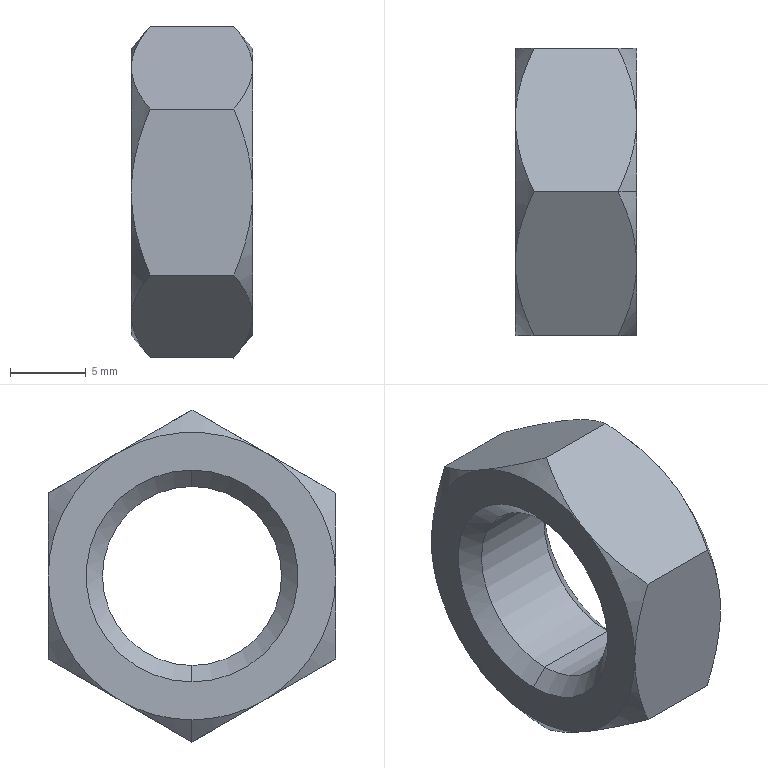Part | SolidWorks | features BaseBody 1 | 1 solid | 28 faces | box 8 x 19 x 21.939 mm | volume 1553 mm3 | cone 18 | plane 8 | cylinder 2 | commonest cylinder face diameters 11.835 x2
STEP:
#1=CARTESIAN_POINT('',(2.917,0.,-5.918));
#2=VERTEX_POINT('',#1);
#3=CARTESIAN_POINT('',(2.917,0.,5.918));
#4=VERTEX_POINT('',#3);
#5=CARTESIAN_POINT('',(2.917,0.,0.));
#6=DIRECTION('',(-1.,0.,0.));
#7=DIRECTION('',(0.,0.,1.));
#8=AXIS2_PLACEMENT_3D('',#5,#6,#7);
#9=CIRCLE('',#8,5.918);
#10=EDGE_CURVE('',#2,#4,#9,.T.);
#11=ORIENTED_EDGE('',*,*,#10,.F.);
#12=CARTESIAN_POINT('',(-2.917,0.,-5.918));
#13=VERTEX_POINT('',#12);
#14=CARTESIAN_POINT('',(4.,0.,-5.918));
#15=DIRECTION('',(-1.,0.,0.));
#16=VECTOR('',#15,1000.);
#17=LINE('',#14,#16);
#18=EDGE_CURVE('',#2,#13,#17,.T.);
#19=ORIENTED_EDGE('',*,*,#18,.T.);
#20=CARTESIAN_POINT('',(-2.917,0.,5.918));
#21=VERTEX_POINT('',#20);
#22=CARTESIAN_POINT('',(-2.917,0.,0.));
#23=DIRECTION('',(1.,0.,0.));
#24=DIRECTION('',(0.,0.,1.));
#25=AXIS2_PLACEMENT_3D('',#22,#23,#24);
#26=CIRCLE('',#25,5.918);
#27=EDGE_CURVE('',#21,#13,#26,.T.);
#28=ORIENTED_EDGE('',*,*,#27,.F.);
#29=CARTESIAN_POINT('',(4.,0.,5.918));
#30=DIRECTION('',(-1.,0.,0.));
#31=VECTOR('',#30,1000.);
#32=LINE('',#29,#31);
#33=EDGE_CURVE('',#4,#21,#32,.T.);
#34=ORIENTED_EDGE('',*,*,#33,.F.);
#35=EDGE_LOOP('',(#11,#19,#28,#34));
#36=FACE_OUTER_BOUND('',#35,.T.);
#37=CARTESIAN_POINT('',(4.,0.,0.));
#38=DIRECTION('',(-1.,0.,0.));
#39=DIRECTION('',(0.,0.,1.));
#40=AXIS2_PLACEMENT_3D('',#37,#38,#39);
#41=CYLINDRICAL_SURFACE('',#40,5.918);
#42=ADVANCED_FACE('',(#36),#41,.F.);
#43=ORIENTED_EDGE('',*,*,#27,.T.);
#44=CARTESIAN_POINT('',(-4.,0.,-7.));
#45=VERTEX_POINT('',#44);
#46=CARTESIAN_POINT('',(-4.,0.,-7.));
#47=DIRECTION('',(-0.7071,0.,-0.7071));
#48=VECTOR('',#47,1000.);
#49=LINE('',#46,#48);
#50=EDGE_CURVE('',#13,#45,#49,.T.);
#51=ORIENTED_EDGE('',*,*,#50,.T.);
#52=CARTESIAN_POINT('',(-4.,0.,7.));
#53=VERTEX_POINT('',#52);
#54=CARTESIAN_POINT('',(-4.,0.,0.));
#55=DIRECTION('',(1.,0.,0.));
#56=DIRECTION('',(0.,0.,1.));
#57=AXIS2_PLACEMENT_3D('',#54,#55,#56);
#58=CIRCLE('',#57,7.);
#59=EDGE_CURVE('',#53,#45,#58,.T.);
#60=ORIENTED_EDGE('',*,*,#59,.F.);
#61=CARTESIAN_POINT('',(-4.,0.,7.));
#62=DIRECTION('',(-0.7071,0.,0.7071));
#63=VECTOR('',#62,1000.);
#64=LINE('',#61,#63);
#65=EDGE_CURVE('',#21,#53,#64,.T.);
#66=ORIENTED_EDGE('',*,*,#65,.F.);
#67=EDGE_LOOP('',(#43,#51,#60,#66));
#68=FACE_OUTER_BOUND('',#67,.T.);
#69=CARTESIAN_POINT('',(-4.,0.,0.));
#70=DIRECTION('',(-1.,0.,0.));
#71=DIRECTION('',(0.,0.,1.));
#72=AXIS2_PLACEMENT_3D('',#69,#70,#71);
#73=CONICAL_SURFACE('',#72,7.,0.7854);
#74=ADVANCED_FACE('',(#68),#73,.F.);
#75=ORIENTED_EDGE('',*,*,#10,.T.);
#76=CARTESIAN_POINT('',(4.,0.,7.));
#77=VERTEX_POINT('',#76);
#78=CARTESIAN_POINT('',(4.,0.,7.));
#79=DIRECTION('',(0.7071,0.,0.7071));
#80=VECTOR('',#79,1000.);
#81=LINE('',#78,#80);
#82=EDGE_CURVE('',#4,#77,#81,.T.);
#83=ORIENTED_EDGE('',*,*,#82,.T.);
#84=CARTESIAN_POINT('',(4.,0.,-7.));
#85=VERTEX_POINT('',#84);
#86=CARTESIAN_POINT('',(4.,0.,0.));
#87=DIRECTION('',(-1.,0.,0.));
#88=DIRECTION('',(0.,0.,-1.));
#89=AXIS2_PLACEMENT_3D('',#86,#87,#88);
#90=CIRCLE('',#89,7.);
#91=EDGE_CURVE('',#85,#77,#90,.T.);
#92=ORIENTED_EDGE('',*,*,#91,.F.);
#93=CARTESIAN_POINT('',(4.,0.,-7.));
#94=DIRECTION('',(0.7071,0.,-0.7071));
#95=VECTOR('',#94,1000.);
#96=LINE('',#93,#95);
#97=EDGE_CURVE('',#2,#85,#96,.T.);
#98=ORIENTED_EDGE('',*,*,#97,.F.);
#99=EDGE_LOOP('',(#75,#83,#92,#98));
#100=FACE_OUTER_BOUND('',#99,.T.);
#101=CARTESIAN_POINT('',(4.,0.,0.));
#102=DIRECTION('',(1.,0.,0.));
#103=DIRECTION('',(0.,0.,-1.));
#104=AXIS2_PLACEMENT_3D('',#101,#102,#103);
#105=CONICAL_SURFACE('',#104,7.,0.7854);
#106=ADVANCED_FACE('',(#100),#105,.F.);
#107=CARTESIAN_POINT('',(-4.,0.,-9.5));
#108=VERTEX_POINT('',#107);
#109=CARTESIAN_POINT('',(-4.,-4.75,-8.227));
#110=VERTEX_POINT('',#109);
#111=CARTESIAN_POINT('',(-4.,0.,0.));
#112=DIRECTION('',(-1.,0.,0.));
#113=DIRECTION('',(0.,0.,-1.));
#114=AXIS2_PLACEMENT_3D('',#111,#112,#113);
#115=CIRCLE('',#114,9.5);
#116=EDGE_CURVE('',#108,#110,#115,.T.);
#117=ORIENTED_EDGE('',*,*,#116,.F.);
#118=CARTESIAN_POINT('',(-2.767,0.000000009,-10.97));
#119=VERTEX_POINT('',#118);
#120=CARTESIAN_POINT('',(-2.759,0.,-10.978));
#121=DIRECTION('',(0.6428,0.,-0.766));
#122=VECTOR('',#121,1000.);
#123=LINE('',#120,#122);
#124=EDGE_CURVE('',#108,#119,#123,.T.);
#125=ORIENTED_EDGE('',*,*,#124,.T.);
#126=CARTESIAN_POINT('',(-2.767,0.000000009,-10.97));
#127=CARTESIAN_POINT('',(-3.503,-1.52,-10.092));
#128=CARTESIAN_POINT('',(-4.,-3.087,-9.188));
#129=CARTESIAN_POINT('',(-4.,-4.75,-8.227));
#130=B_SPLINE_CURVE_WITH_KNOTS('',3,(#126,#127,#128,#129),.UNSPECIFIED.,.F.,.F.,(4,4),(0.,0.005622),.UNSPECIFIED.);
#131=EDGE_CURVE('',#119,#110,#130,.T.);
#132=ORIENTED_EDGE('',*,*,#131,.T.);
#133=EDGE_LOOP('',(#117,#125,#132));
#134=FACE_OUTER_BOUND('',#133,.T.);
#135=CARTESIAN_POINT('',(-2.759,0.,0.));
#136=DIRECTION('',(1.,0.,0.));
#137=DIRECTION('',(0.,0.,-1.));
#138=AXIS2_PLACEMENT_3D('',#135,#136,#137);
#139=CONICAL_SURFACE('',#138,10.978,0.8727);
#140=ADVANCED_FACE('',(#134),#139,.T.);
#141=CARTESIAN_POINT('',(4.,0.,9.5));
#142=VERTEX_POINT('',#141);
#143=CARTESIAN_POINT('',(4.,-4.75,8.227));
#144=VERTEX_POINT('',#143);
#145=CARTESIAN_POINT('',(4.,0.,0.));
#146=DIRECTION('',(1.,0.,0.));
#147=DIRECTION('',(0.,0.,1.));
#148=AXIS2_PLACEMENT_3D('',#145,#146,#147);
#149=CIRCLE('',#148,9.5);
#150=EDGE_CURVE('',#142,#144,#149,.T.);
#151=ORIENTED_EDGE('',*,*,#150,.F.);
#152=CARTESIAN_POINT('',(2.767,0.000000009,10.97));
#153=VERTEX_POINT('',#152);
#154=CARTESIAN_POINT('',(2.759,0.,10.978));
#155=DIRECTION('',(-0.6428,0.,0.766));
#156=VECTOR('',#155,1000.);
#157=LINE('',#154,#156);
#158=EDGE_CURVE('',#142,#153,#157,.T.);
#159=ORIENTED_EDGE('',*,*,#158,.T.);
#160=CARTESIAN_POINT('',(2.767,0.000000009,10.97));
#161=CARTESIAN_POINT('',(3.503,-1.52,10.092));
#162=CARTESIAN_POINT('',(4.,-3.087,9.188));
#163=CARTESIAN_POINT('',(4.,-4.75,8.227));
#164=B_SPLINE_CURVE_WITH_KNOTS('',3,(#160,#161,#162,#163),.UNSPECIFIED.,.F.,.F.,(4,4),(0.,0.005622),.UNSPECIFIED.);
#165=EDGE_CURVE('',#153,#144,#164,.T.);
#166=ORIENTED_EDGE('',*,*,#165,.T.);
#167=EDGE_LOOP('',(#151,#159,#166));
#168=FACE_OUTER_BOUND('',#167,.T.);
#169=CARTESIAN_POINT('',(2.759,0.,0.));
#170=DIRECTION('',(-1.,0.,0.));
#171=DIRECTION('',(0.,0.,1.));
#172=AXIS2_PLACEMENT_3D('',#169,#170,#171);
#173=CONICAL_SURFACE('',#172,10.978,0.8727);
#174=ADVANCED_FACE('',(#168),#173,.T.);
#175=ORIENTED_EDGE('',*,*,#18,.F.);
#176=CARTESIAN_POINT('',(2.917,0.,0.));
#177=DIRECTION('',(-1.,0.,0.));
#178=DIRECTION('',(0.,0.,1.));
#179=AXIS2_PLACEMENT_3D('',#176,#177,#178);
#180=CIRCLE('',#179,5.918);
#181=EDGE_CURVE('',#4,#2,#180,.T.);
#182=ORIENTED_EDGE('',*,*,#181,.F.);
#183=ORIENTED_EDGE('',*,*,#33,.T.);
#184=CARTESIAN_POINT('',(-2.917,0.,0.));
#185=DIRECTION('',(1.,0.,0.));
#186=DIRECTION('',(0.,0.,1.));
#187=AXIS2_PLACEMENT_3D('',#184,#185,#186);
#188=CIRCLE('',#187,5.918);
#189=EDGE_CURVE('',#13,#21,#188,.T.);
#190=ORIENTED_EDGE('',*,*,#189,.F.);
#191=EDGE_LOOP('',(#175,#182,#183,#190));
#192=FACE_OUTER_BOUND('',#191,.T.);
#193=CARTESIAN_POINT('',(4.,0.,0.));
#194=DIRECTION('',(-1.,0.,0.));
#195=DIRECTION('',(0.,0.,1.));
#196=AXIS2_PLACEMENT_3D('',#193,#194,#195);
#197=CYLINDRICAL_SURFACE('',#196,5.918);
#198=ADVANCED_FACE('',(#192),#197,.F.);
#199=ORIENTED_EDGE('',*,*,#50,.F.);
#200=ORIENTED_EDGE('',*,*,#189,.T.);
#201=ORIENTED_EDGE('',*,*,#65,.T.);
#202=CARTESIAN_POINT('',(-4.,0.,0.));
#203=DIRECTION('',(1.,0.,0.));
#204=DIRECTION('',(0.,0.,1.));
#205=AXIS2_PLACEMENT_3D('',#202,#203,#204);
#206=CIRCLE('',#205,7.);
#207=EDGE_CURVE('',#45,#53,#206,.T.);
#208=ORIENTED_EDGE('',*,*,#207,.F.);
#209=EDGE_LOOP('',(#199,#200,#201,#208));
#210=FACE_OUTER_BOUND('',#209,.T.);
#211=CARTESIAN_POINT('',(-4.,0.,0.));
#212=DIRECTION('',(-1.,0.,0.));
#213=DIRECTION('',(0.,0.,1.));
#214=AXIS2_PLACEMENT_3D('',#211,#212,#213);
#215=CONICAL_SURFACE('',#214,7.,0.7854);
#216=ADVANCED_FACE('',(#210),#215,.F.);
#217=ORIENTED_EDGE('',*,*,#82,.F.);
#218=ORIENTED_EDGE('',*,*,#181,.T.);
#219=ORIENTED_EDGE('',*,*,#97,.T.);
#220=CARTESIAN_POINT('',(4.,0.,0.));
#221=DIRECTION('',(-1.,0.,0.));
#222=DIRECTION('',(0.,0.,-1.));
#223=AXIS2_PLACEMENT_3D('',#220,#221,#222);
#224=CIRCLE('',#223,7.);
#225=EDGE_CURVE('',#77,#85,#224,.T.);
#226=ORIENTED_EDGE('',*,*,#225,.F.);
#227=EDGE_LOOP('',(#217,#218,#219,#226));
#228=FACE_OUTER_BOUND('',#227,.T.);
#229=CARTESIAN_POINT('',(4.,0.,0.));
#230=DIRECTION('',(1.,0.,0.));
#231=DIRECTION('',(0.,0.,-1.));
#232=AXIS2_PLACEMENT_3D('',#229,#230,#231);
#233=CONICAL_SURFACE('',#232,7.,0.7854);
#234=ADVANCED_FACE('',(#228),#233,.F.);
#235=CARTESIAN_POINT('',(-4.,-9.5,0.));
#236=VERTEX_POINT('',#235);
#237=CARTESIAN_POINT('',(-4.,-4.75,8.227));
#238=VERTEX_POINT('',#237);
#239=CARTESIAN_POINT('',(-4.,0.,0.));
#240=DIRECTION('',(-1.,0.,0.));
#241=DIRECTION('',(0.,1.,0.));
#242=AXIS2_PLACEMENT_3D('',#239,#240,#241);
#243=CIRCLE('',#242,9.5);
#244=EDGE_CURVE('',#236,#238,#243,.T.);
#245=ORIENTED_EDGE('',*,*,#244,.T.);
#246=CARTESIAN_POINT('',(-4.,4.75,8.227));
#247=VERTEX_POINT('',#246);
#248=CARTESIAN_POINT('',(-4.,0.,0.));
#249=DIRECTION('',(-1.,0.,0.));
#250=DIRECTION('',(0.,0.,-1.));
#251=AXIS2_PLACEMENT_3D('',#248,#249,#250);
#252=CIRCLE('',#251,9.5);
#253=EDGE_CURVE('',#238,#247,#252,.T.);
#254=ORIENTED_EDGE('',*,*,#253,.T.);
#255=CARTESIAN_POINT('',(-4.,9.5,0.));
#256=VERTEX_POINT('',#255);
#257=CARTESIAN_POINT('',(-4.,0.,0.));
#258=DIRECTION('',(-1.,0.,0.));
#259=DIRECTION('',(0.,0.,-1.));
#260=AXIS2_PLACEMENT_3D('',#257,#258,#259);
#261=CIRCLE('',#260,9.5);
#262=EDGE_CURVE('',#247,#256,#261,.T.);
#263=ORIENTED_EDGE('',*,*,#262,.T.);
#264=CARTESIAN_POINT('',(-4.,4.75,-8.227));
#265=VERTEX_POINT('',#264);
#266=CARTESIAN_POINT('',(-4.,0.,0.));
#267=DIRECTION('',(-1.,0.,0.));
#268=DIRECTION('',(0.,1.,0.));
#269=AXIS2_PLACEMENT_3D('',#266,#267,#268);
#270=CIRCLE('',#269,9.5);
#271=EDGE_CURVE('',#256,#265,#270,.T.);
#272=ORIENTED_EDGE('',*,*,#271,.T.);
#273=CARTESIAN_POINT('',(-4.,0.,0.));
#274=DIRECTION('',(-1.,0.,0.));
#275=DIRECTION('',(0.,0.,-1.));
#276=AXIS2_PLACEMENT_3D('',#273,#274,#275);
#277=CIRCLE('',#276,9.5);
#278=EDGE_CURVE('',#265,#108,#277,.T.);
#279=ORIENTED_EDGE('',*,*,#278,.T.);
#280=ORIENTED_EDGE('',*,*,#116,.T.);
#281=CARTESIAN_POINT('',(-4.,0.,0.));
#282=DIRECTION('',(-1.,0.,0.));
#283=DIRECTION('',(0.,0.,-1.));
#284=AXIS2_PLACEMENT_3D('',#281,#282,#283);
#285=CIRCLE('',#284,9.5);
#286=EDGE_CURVE('',#110,#236,#285,.T.);
#287=ORIENTED_EDGE('',*,*,#286,.T.);
#288=EDGE_LOOP('',(#245,#254,#263,#272,#279,#280,#287));
#289=FACE_OUTER_BOUND('',#288,.T.);
#290=ORIENTED_EDGE('',*,*,#59,.T.);
#291=ORIENTED_EDGE('',*,*,#207,.T.);
#292=EDGE_LOOP('',(#290,#291));
#293=FACE_BOUND('',#292,.T.);
#294=CARTESIAN_POINT('',(-4.,9.5,0.));
#295=DIRECTION('',(-1.,0.,0.));
#296=DIRECTION('',(0.,0.,1.));
#297=AXIS2_PLACEMENT_3D('',#294,#295,#296);
#298=PLANE('',#297);
#299=ADVANCED_FACE('',(#289,#293),#298,.T.);
#300=ORIENTED_EDGE('',*,*,#91,.T.);
#301=ORIENTED_EDGE('',*,*,#225,.T.);
#302=EDGE_LOOP('',(#300,#301));
#303=FACE_BOUND('',#302,.T.);
#304=CARTESIAN_POINT('',(4.,-9.5,0.));
#305=VERTEX_POINT('',#304);
#306=CARTESIAN_POINT('',(4.,-4.75,-8.227));
#307=VERTEX_POINT('',#306);
#308=CARTESIAN_POINT('',(4.,0.,0.));
#309=DIRECTION('',(1.,0.,0.));
#310=DIRECTION('',(0.,0.,1.));
#311=AXIS2_PLACEMENT_3D('',#308,#309,#310);
#312=CIRCLE('',#311,9.5);
#313=EDGE_CURVE('',#305,#307,#312,.T.);
#314=ORIENTED_EDGE('',*,*,#313,.T.);
#315=CARTESIAN_POINT('',(4.,4.75,-8.227));
#316=VERTEX_POINT('',#315);
#317=CARTESIAN_POINT('',(4.,0.,0.));
#318=DIRECTION('',(1.,0.,0.));
#319=DIRECTION('',(0.,0.,1.));
#320=AXIS2_PLACEMENT_3D('',#317,#318,#319);
#321=CIRCLE('',#320,9.5);
#322=EDGE_CURVE('',#307,#316,#321,.T.);
#323=ORIENTED_EDGE('',*,*,#322,.T.);
#324=CARTESIAN_POINT('',(4.,9.5,0.));
#325=VERTEX_POINT('',#324);
#326=CARTESIAN_POINT('',(4.,0.,0.));
#327=DIRECTION('',(1.,0.,0.));
#328=DIRECTION('',(0.,0.,1.));
#329=AXIS2_PLACEMENT_3D('',#326,#327,#328);
#330=CIRCLE('',#329,9.5);
#331=EDGE_CURVE('',#316,#325,#330,.T.);
#332=ORIENTED_EDGE('',*,*,#331,.T.);
#333=CARTESIAN_POINT('',(4.,4.75,8.227));
#334=VERTEX_POINT('',#333);
#335=CARTESIAN_POINT('',(4.,0.,0.));
#336=DIRECTION('',(1.,0.,0.));
#337=DIRECTION('',(0.,0.,1.));
#338=AXIS2_PLACEMENT_3D('',#335,#336,#337);
#339=CIRCLE('',#338,9.5);
#340=EDGE_CURVE('',#325,#334,#339,.T.);
#341=ORIENTED_EDGE('',*,*,#340,.T.);
#342=CARTESIAN_POINT('',(4.,0.,0.));
#343=DIRECTION('',(1.,0.,0.));
#344=DIRECTION('',(0.,0.,1.));
#345=AXIS2_PLACEMENT_3D('',#342,#343,#344);
#346=CIRCLE('',#345,9.5);
#347=EDGE_CURVE('',#334,#142,#346,.T.);
#348=ORIENTED_EDGE('',*,*,#347,.T.);
#349=ORIENTED_EDGE('',*,*,#150,.T.);
#350=CARTESIAN_POINT('',(4.,0.,0.));
#351=DIRECTION('',(1.,0.,0.));
#352=DIRECTION('',(0.,0.,1.));
#353=AXIS2_PLACEMENT_3D('',#350,#351,#352);
#354=CIRCLE('',#353,9.5);
#355=EDGE_CURVE('',#144,#305,#354,.T.);
#356=ORIENTED_EDGE('',*,*,#355,.T.);
#357=EDGE_LOOP('',(#314,#323,#332,#341,#348,#349,#356));
#358=FACE_OUTER_BOUND('',#357,.T.);
#359=CARTESIAN_POINT('',(4.,7.,0.));
#360=DIRECTION('',(1.,0.,0.));
#361=DIRECTION('',(0.,0.,-1.));
#362=AXIS2_PLACEMENT_3D('',#359,#360,#361);
#363=PLANE('',#362);
#364=ADVANCED_FACE('',(#303,#358),#363,.T.);
#365=ORIENTED_EDGE('',*,*,#253,.F.);
#366=CARTESIAN_POINT('',(-2.767,0.000000018,10.97));
#367=VERTEX_POINT('',#366);
#368=CARTESIAN_POINT('',(-4.,-4.75,8.227));
#369=CARTESIAN_POINT('',(-4.,-3.926,8.703));
#370=CARTESIAN_POINT('',(-3.879,-3.12,9.168));
#371=CARTESIAN_POINT('',(-3.445,-1.537,10.083));
#372=CARTESIAN_POINT('',(-3.134,-0.7569,10.533));
#373=CARTESIAN_POINT('',(-2.767,0.000000018,10.97));
#374=B_SPLINE_CURVE_WITH_KNOTS('',3,(#368,#369,#370,#371,#372,#373),.UNSPECIFIED.,.F.,.F.,(4,2,4),(0.,0.002813,0.005627),.UNSPECIFIED.);
#375=EDGE_CURVE('',#238,#367,#374,.T.);
#376=ORIENTED_EDGE('',*,*,#375,.T.);
#377=CARTESIAN_POINT('',(-2.767,0.000000018,10.97));
#378=CARTESIAN_POINT('',(-3.503,1.52,10.092));
#379=CARTESIAN_POINT('',(-4.,3.087,9.188));
#380=CARTESIAN_POINT('',(-4.,4.75,8.227));
#381=B_SPLINE_CURVE_WITH_KNOTS('',3,(#377,#378,#379,#380),.UNSPECIFIED.,.F.,.F.,(4,4),(0.,0.005622),.UNSPECIFIED.);
#382=EDGE_CURVE('',#367,#247,#381,.T.);
#383=ORIENTED_EDGE('',*,*,#382,.T.);
#384=EDGE_LOOP('',(#365,#376,#383));
#385=FACE_OUTER_BOUND('',#384,.T.);
#386=CARTESIAN_POINT('',(-2.759,0.,0.));
#387=DIRECTION('',(1.,0.,0.));
#388=DIRECTION('',(0.,0.,-1.));
#389=AXIS2_PLACEMENT_3D('',#386,#387,#388);
#390=CONICAL_SURFACE('',#389,10.978,0.8727);
#391=ADVANCED_FACE('',(#385),#390,.T.);
#392=CARTESIAN_POINT('',(-2.767,-9.5,5.485));
#393=VERTEX_POINT('',#392);
#394=CARTESIAN_POINT('',(-2.767,-9.5,5.485));
#395=CARTESIAN_POINT('',(-3.503,-7.98,6.362));
#396=CARTESIAN_POINT('',(-4.,-6.413,7.267));
#397=CARTESIAN_POINT('',(-4.,-4.75,8.227));
#398=B_SPLINE_CURVE_WITH_KNOTS('',3,(#394,#395,#396,#397),.UNSPECIFIED.,.F.,.F.,(4,4),(0.,0.005622),.UNSPECIFIED.);
#399=EDGE_CURVE('',#393,#238,#398,.T.);
#400=ORIENTED_EDGE('',*,*,#399,.T.);
#401=ORIENTED_EDGE('',*,*,#244,.F.);
#402=CARTESIAN_POINT('',(-4.,-9.5,0.));
#403=CARTESIAN_POINT('',(-4.,-9.5,0.9511));
#404=CARTESIAN_POINT('',(-3.879,-9.5,1.882));
#405=CARTESIAN_POINT('',(-3.445,-9.5,3.711));
#406=CARTESIAN_POINT('',(-3.134,-9.5,4.611));
#407=CARTESIAN_POINT('',(-2.767,-9.5,5.485));
#408=B_SPLINE_CURVE_WITH_KNOTS('',3,(#402,#403,#404,#405,#406,#407),.UNSPECIFIED.,.F.,.F.,(4,2,4),(0.,0.002813,0.005627),.UNSPECIFIED.);
#409=EDGE_CURVE('',#236,#393,#408,.T.);
#410=ORIENTED_EDGE('',*,*,#409,.T.);
#411=EDGE_LOOP('',(#400,#401,#410));
#412=FACE_OUTER_BOUND('',#411,.T.);
#413=CARTESIAN_POINT('',(-2.759,0.,0.));
#414=DIRECTION('',(1.,0.,0.));
#415=DIRECTION('',(0.,1.,0.));
#416=AXIS2_PLACEMENT_3D('',#413,#414,#415);
#417=CONICAL_SURFACE('',#416,10.978,0.8727);
#418=ADVANCED_FACE('',(#412),#417,.T.);
#419=CARTESIAN_POINT('',(-2.767,-9.5,-5.485));
#420=VERTEX_POINT('',#419);
#421=CARTESIAN_POINT('',(-2.767,-9.5,-5.485));
#422=CARTESIAN_POINT('',(-3.503,-9.5,-3.73));
#423=CARTESIAN_POINT('',(-4.,-9.5,-1.921));
#424=CARTESIAN_POINT('',(-4.,-9.5,0.));
#425=B_SPLINE_CURVE_WITH_KNOTS('',3,(#421,#422,#423,#424),.UNSPECIFIED.,.F.,.F.,(4,4),(0.,0.005622),.UNSPECIFIED.);
#426=EDGE_CURVE('',#420,#236,#425,.T.);
#427=ORIENTED_EDGE('',*,*,#426,.T.);
#428=ORIENTED_EDGE('',*,*,#286,.F.);
#429=CARTESIAN_POINT('',(-4.,-4.75,-8.227));
#430=CARTESIAN_POINT('',(-4.,-5.574,-7.752));
#431=CARTESIAN_POINT('',(-3.879,-6.38,-7.286));
#432=CARTESIAN_POINT('',(-3.445,-7.963,-6.372));
#433=CARTESIAN_POINT('',(-3.134,-8.743,-5.922));
#434=CARTESIAN_POINT('',(-2.767,-9.5,-5.485));
#435=B_SPLINE_CURVE_WITH_KNOTS('',3,(#429,#430,#431,#432,#433,#434),.UNSPECIFIED.,.F.,.F.,(4,2,4),(0.,0.002813,0.005627),.UNSPECIFIED.);
#436=EDGE_CURVE('',#110,#420,#435,.T.);
#437=ORIENTED_EDGE('',*,*,#436,.T.);
#438=EDGE_LOOP('',(#427,#428,#437));
#439=FACE_OUTER_BOUND('',#438,.T.);
#440=CARTESIAN_POINT('',(-2.759,0.,0.));
#441=DIRECTION('',(1.,0.,0.));
#442=DIRECTION('',(0.,0.,-1.));
#443=AXIS2_PLACEMENT_3D('',#440,#441,#442);
#444=CONICAL_SURFACE('',#443,10.978,0.8727);
#445=ADVANCED_FACE('',(#439),#444,.T.);
#446=ORIENTED_EDGE('',*,*,#124,.F.);
#447=ORIENTED_EDGE('',*,*,#278,.F.);
#448=CARTESIAN_POINT('',(-4.,4.75,-8.227));
#449=CARTESIAN_POINT('',(-4.,3.926,-8.703));
#450=CARTESIAN_POINT('',(-3.879,3.12,-9.168));
#451=CARTESIAN_POINT('',(-3.445,1.537,-10.083));
#452=CARTESIAN_POINT('',(-3.134,0.7569,-10.533));
#453=CARTESIAN_POINT('',(-2.767,0.000000009,-10.97));
#454=B_SPLINE_CURVE_WITH_KNOTS('',3,(#448,#449,#450,#451,#452,#453),.UNSPECIFIED.,.F.,.F.,(4,2,4),(0.,0.002813,0.005627),.UNSPECIFIED.);
#455=EDGE_CURVE('',#265,#119,#454,.T.);
#456=ORIENTED_EDGE('',*,*,#455,.T.);
#457=EDGE_LOOP('',(#446,#447,#456));
#458=FACE_OUTER_BOUND('',#457,.T.);
#459=CARTESIAN_POINT('',(-2.759,0.,0.));
#460=DIRECTION('',(1.,0.,0.));
#461=DIRECTION('',(0.,0.,-1.));
#462=AXIS2_PLACEMENT_3D('',#459,#460,#461);
#463=CONICAL_SURFACE('',#462,10.978,0.8727);
#464=ADVANCED_FACE('',(#458),#463,.T.);
#465=ORIENTED_EDGE('',*,*,#271,.F.);
#466=CARTESIAN_POINT('',(-2.767,9.5,-5.485));
#467=VERTEX_POINT('',#466);
#468=CARTESIAN_POINT('',(-4.,9.5,0.));
#469=CARTESIAN_POINT('',(-4.,9.5,-0.9511));
#470=CARTESIAN_POINT('',(-3.879,9.5,-1.882));
#471=CARTESIAN_POINT('',(-3.445,9.5,-3.711));
#472=CARTESIAN_POINT('',(-3.134,9.5,-4.611));
#473=CARTESIAN_POINT('',(-2.767,9.5,-5.485));
#474=B_SPLINE_CURVE_WITH_KNOTS('',3,(#468,#469,#470,#471,#472,#473),.UNSPECIFIED.,.F.,.F.,(4,2,4),(0.,0.002813,0.005627),.UNSPECIFIED.);
#475=EDGE_CURVE('',#256,#467,#474,.T.);
#476=ORIENTED_EDGE('',*,*,#475,.T.);
#477=CARTESIAN_POINT('',(-2.767,9.5,-5.485));
#478=CARTESIAN_POINT('',(-3.503,7.98,-6.362));
#479=CARTESIAN_POINT('',(-4.,6.413,-7.267));
#480=CARTESIAN_POINT('',(-4.,4.75,-8.227));
#481=B_SPLINE_CURVE_WITH_KNOTS('',3,(#477,#478,#479,#480),.UNSPECIFIED.,.F.,.F.,(4,4),(0.,0.005622),.UNSPECIFIED.);
#482=EDGE_CURVE('',#467,#265,#481,.T.);
#483=ORIENTED_EDGE('',*,*,#482,.T.);
#484=EDGE_LOOP('',(#465,#476,#483));
#485=FACE_OUTER_BOUND('',#484,.T.);
#486=CARTESIAN_POINT('',(-2.759,0.,0.));
#487=DIRECTION('',(1.,0.,0.));
#488=DIRECTION('',(0.,1.,0.));
#489=AXIS2_PLACEMENT_3D('',#486,#487,#488);
#490=CONICAL_SURFACE('',#489,10.978,0.8727);
#491=ADVANCED_FACE('',(#485),#490,.T.);
#492=ORIENTED_EDGE('',*,*,#262,.F.);
#493=CARTESIAN_POINT('',(-2.767,9.5,5.485));
#494=VERTEX_POINT('',#493);
#495=CARTESIAN_POINT('',(-4.,4.75,8.227));
#496=CARTESIAN_POINT('',(-4.,5.574,7.752));
#497=CARTESIAN_POINT('',(-3.879,6.38,7.286));
#498=CARTESIAN_POINT('',(-3.445,7.963,6.372));
#499=CARTESIAN_POINT('',(-3.134,8.743,5.922));
#500=CARTESIAN_POINT('',(-2.767,9.5,5.485));
#501=B_SPLINE_CURVE_WITH_KNOTS('',3,(#495,#496,#497,#498,#499,#500),.UNSPECIFIED.,.F.,.F.,(4,2,4),(0.,0.002813,0.005627),.UNSPECIFIED.);
#502=EDGE_CURVE('',#247,#494,#501,.T.);
#503=ORIENTED_EDGE('',*,*,#502,.T.);
#504=CARTESIAN_POINT('',(-2.767,9.5,5.485));
#505=CARTESIAN_POINT('',(-3.503,9.5,3.73));
#506=CARTESIAN_POINT('',(-4.,9.5,1.921));
#507=CARTESIAN_POINT('',(-4.,9.5,0.));
#508=B_SPLINE_CURVE_WITH_KNOTS('',3,(#504,#505,#506,#507),.UNSPECIFIED.,.F.,.F.,(4,4),(0.,0.005622),.UNSPECIFIED.);
#509=EDGE_CURVE('',#494,#256,#508,.T.);
#510=ORIENTED_EDGE('',*,*,#509,.T.);
#511=EDGE_LOOP('',(#492,#503,#510));
#512=FACE_OUTER_BOUND('',#511,.T.);
#513=CARTESIAN_POINT('',(-2.759,0.,0.));
#514=DIRECTION('',(1.,0.,0.));
#515=DIRECTION('',(0.,0.,-1.));
#516=AXIS2_PLACEMENT_3D('',#513,#514,#515);
#517=CONICAL_SURFACE('',#516,10.978,0.8727);
#518=ADVANCED_FACE('',(#512),#517,.T.);
#519=ORIENTED_EDGE('',*,*,#322,.F.);
#520=CARTESIAN_POINT('',(2.767,0.000000018,-10.97));
#521=VERTEX_POINT('',#520);
#522=CARTESIAN_POINT('',(4.,-4.75,-8.227));
#523=CARTESIAN_POINT('',(4.,-3.926,-8.703));
#524=CARTESIAN_POINT('',(3.879,-3.12,-9.168));
#525=CARTESIAN_POINT('',(3.445,-1.537,-10.083));
#526=CARTESIAN_POINT('',(3.134,-0.7569,-10.533));
#527=CARTESIAN_POINT('',(2.767,0.000000018,-10.97));
#528=B_SPLINE_CURVE_WITH_KNOTS('',3,(#522,#523,#524,#525,#526,#527),.UNSPECIFIED.,.F.,.F.,(4,2,4),(0.,0.002813,0.005627),.UNSPECIFIED.);
#529=EDGE_CURVE('',#307,#521,#528,.T.);
#530=ORIENTED_EDGE('',*,*,#529,.T.);
#531=CARTESIAN_POINT('',(2.767,0.000000018,-10.97));
#532=CARTESIAN_POINT('',(3.503,1.52,-10.092));
#533=CARTESIAN_POINT('',(4.,3.087,-9.188));
#534=CARTESIAN_POINT('',(4.,4.75,-8.227));
#535=B_SPLINE_CURVE_WITH_KNOTS('',3,(#531,#532,#533,#534),.UNSPECIFIED.,.F.,.F.,(4,4),(0.,0.005622),.UNSPECIFIED.);
#536=EDGE_CURVE('',#521,#316,#535,.T.);
#537=ORIENTED_EDGE('',*,*,#536,.T.);
#538=EDGE_LOOP('',(#519,#530,#537));
#539=FACE_OUTER_BOUND('',#538,.T.);
#540=CARTESIAN_POINT('',(2.759,0.,0.));
#541=DIRECTION('',(-1.,0.,0.));
#542=DIRECTION('',(0.,0.,1.));
#543=AXIS2_PLACEMENT_3D('',#540,#541,#542);
#544=CONICAL_SURFACE('',#543,10.978,0.8727);
#545=ADVANCED_FACE('',(#539),#544,.T.);
#546=ORIENTED_EDGE('',*,*,#313,.F.);
#547=CARTESIAN_POINT('',(2.767,-9.5,-5.485));
#548=VERTEX_POINT('',#547);
#549=CARTESIAN_POINT('',(4.,-9.5,0.));
#550=CARTESIAN_POINT('',(4.,-9.5,-0.9511));
#551=CARTESIAN_POINT('',(3.879,-9.5,-1.882));
#552=CARTESIAN_POINT('',(3.445,-9.5,-3.711));
#553=CARTESIAN_POINT('',(3.134,-9.5,-4.611));
#554=CARTESIAN_POINT('',(2.767,-9.5,-5.485));
#555=B_SPLINE_CURVE_WITH_KNOTS('',3,(#549,#550,#551,#552,#553,#554),.UNSPECIFIED.,.F.,.F.,(4,2,4),(0.,0.002813,0.005627),.UNSPECIFIED.);
#556=EDGE_CURVE('',#305,#548,#555,.T.);
#557=ORIENTED_EDGE('',*,*,#556,.T.);
#558=CARTESIAN_POINT('',(2.767,-9.5,-5.485));
#559=CARTESIAN_POINT('',(3.503,-7.98,-6.362));
#560=CARTESIAN_POINT('',(4.,-6.413,-7.267));
#561=CARTESIAN_POINT('',(4.,-4.75,-8.227));
#562=B_SPLINE_CURVE_WITH_KNOTS('',3,(#558,#559,#560,#561),.UNSPECIFIED.,.F.,.F.,(4,4),(0.,0.005622),.UNSPECIFIED.);
#563=EDGE_CURVE('',#548,#307,#562,.T.);
#564=ORIENTED_EDGE('',*,*,#563,.T.);
#565=EDGE_LOOP('',(#546,#557,#564));
#566=FACE_OUTER_BOUND('',#565,.T.);
#567=CARTESIAN_POINT('',(2.759,0.,0.));
#568=DIRECTION('',(-1.,0.,0.));
#569=DIRECTION('',(0.,0.,1.));
#570=AXIS2_PLACEMENT_3D('',#567,#568,#569);
#571=CONICAL_SURFACE('',#570,10.978,0.8727);
#572=ADVANCED_FACE('',(#566),#571,.T.);
#573=ORIENTED_EDGE('',*,*,#355,.F.);
#574=CARTESIAN_POINT('',(2.767,-9.5,5.485));
#575=VERTEX_POINT('',#574);
#576=CARTESIAN_POINT('',(4.,-4.75,8.227));
#577=CARTESIAN_POINT('',(4.,-5.574,7.752));
#578=CARTESIAN_POINT('',(3.879,-6.38,7.286));
#579=CARTESIAN_POINT('',(3.445,-7.963,6.372));
#580=CARTESIAN_POINT('',(3.134,-8.743,5.922));
#581=CARTESIAN_POINT('',(2.767,-9.5,5.485));
#582=B_SPLINE_CURVE_WITH_KNOTS('',3,(#576,#577,#578,#579,#580,#581),.UNSPECIFIED.,.F.,.F.,(4,2,4),(0.,0.002813,0.005627),.UNSPECIFIED.);
#583=EDGE_CURVE('',#144,#575,#582,.T.);
#584=ORIENTED_EDGE('',*,*,#583,.T.);
#585=CARTESIAN_POINT('',(2.767,-9.5,5.485));
#586=CARTESIAN_POINT('',(3.503,-9.5,3.73));
#587=CARTESIAN_POINT('',(4.,-9.5,1.921));
#588=CARTESIAN_POINT('',(4.,-9.5,0.));
#589=B_SPLINE_CURVE_WITH_KNOTS('',3,(#585,#586,#587,#588),.UNSPECIFIED.,.F.,.F.,(4,4),(0.,0.005622),.UNSPECIFIED.);
#590=EDGE_CURVE('',#575,#305,#589,.T.);
#591=ORIENTED_EDGE('',*,*,#590,.T.);
#592=EDGE_LOOP('',(#573,#584,#591));
#593=FACE_OUTER_BOUND('',#592,.T.);
#594=CARTESIAN_POINT('',(2.759,0.,0.));
#595=DIRECTION('',(-1.,0.,0.));
#596=DIRECTION('',(0.,0.,1.));
#597=AXIS2_PLACEMENT_3D('',#594,#595,#596);
#598=CONICAL_SURFACE('',#597,10.978,0.8727);
#599=ADVANCED_FACE('',(#593),#598,.T.);
#600=ORIENTED_EDGE('',*,*,#158,.F.);
#601=ORIENTED_EDGE('',*,*,#347,.F.);
#602=CARTESIAN_POINT('',(4.,4.75,8.227));
#603=CARTESIAN_POINT('',(4.,3.926,8.703));
#604=CARTESIAN_POINT('',(3.879,3.12,9.168));
#605=CARTESIAN_POINT('',(3.445,1.537,10.083));
#606=CARTESIAN_POINT('',(3.134,0.7569,10.533));
#607=CARTESIAN_POINT('',(2.767,0.000000009,10.97));
#608=B_SPLINE_CURVE_WITH_KNOTS('',3,(#602,#603,#604,#605,#606,#607),.UNSPECIFIED.,.F.,.F.,(4,2,4),(0.,0.002813,0.005627),.UNSPECIFIED.);
#609=EDGE_CURVE('',#334,#153,#608,.T.);
#610=ORIENTED_EDGE('',*,*,#609,.T.);
#611=EDGE_LOOP('',(#600,#601,#610));
#612=FACE_OUTER_BOUND('',#611,.T.);
#613=CARTESIAN_POINT('',(2.759,0.,0.));
#614=DIRECTION('',(-1.,0.,0.));
#615=DIRECTION('',(0.,0.,1.));
#616=AXIS2_PLACEMENT_3D('',#613,#614,#615);
#617=CONICAL_SURFACE('',#616,10.978,0.8727);
#618=ADVANCED_FACE('',(#612),#617,.T.);
#619=ORIENTED_EDGE('',*,*,#340,.F.);
#620=CARTESIAN_POINT('',(2.767,9.5,5.485));
#621=VERTEX_POINT('',#620);
#622=CARTESIAN_POINT('',(4.,9.5,0.));
#623=CARTESIAN_POINT('',(4.,9.5,0.9511));
#624=CARTESIAN_POINT('',(3.879,9.5,1.882));
#625=CARTESIAN_POINT('',(3.445,9.5,3.711));
#626=CARTESIAN_POINT('',(3.134,9.5,4.611));
#627=CARTESIAN_POINT('',(2.767,9.5,5.485));
#628=B_SPLINE_CURVE_WITH_KNOTS('',3,(#622,#623,#624,#625,#626,#627),.UNSPECIFIED.,.F.,.F.,(4,2,4),(0.,0.002813,0.005627),.UNSPECIFIED.);
#629=EDGE_CURVE('',#325,#621,#628,.T.);
#630=ORIENTED_EDGE('',*,*,#629,.T.);
#631=CARTESIAN_POINT('',(2.767,9.5,5.485));
#632=CARTESIAN_POINT('',(3.503,7.98,6.362));
#633=CARTESIAN_POINT('',(4.,6.413,7.267));
#634=CARTESIAN_POINT('',(4.,4.75,8.227));
#635=B_SPLINE_CURVE_WITH_KNOTS('',3,(#631,#632,#633,#634),.UNSPECIFIED.,.F.,.F.,(4,4),(0.,0.005622),.UNSPECIFIED.);
#636=EDGE_CURVE('',#621,#334,#635,.T.);
#637=ORIENTED_EDGE('',*,*,#636,.T.);
#638=EDGE_LOOP('',(#619,#630,#637));
#639=FACE_OUTER_BOUND('',#638,.T.);
#640=CARTESIAN_POINT('',(2.759,0.,0.));
#641=DIRECTION('',(-1.,0.,0.));
#642=DIRECTION('',(0.,0.,1.));
#643=AXIS2_PLACEMENT_3D('',#640,#641,#642);
#644=CONICAL_SURFACE('',#643,10.978,0.8727);
#645=ADVANCED_FACE('',(#639),#644,.T.);
#646=ORIENTED_EDGE('',*,*,#331,.F.);
#647=CARTESIAN_POINT('',(2.767,9.5,-5.485));
#648=VERTEX_POINT('',#647);
#649=CARTESIAN_POINT('',(4.,4.75,-8.227));
#650=CARTESIAN_POINT('',(4.,5.574,-7.752));
#651=CARTESIAN_POINT('',(3.879,6.38,-7.286));
#652=CARTESIAN_POINT('',(3.445,7.963,-6.372));
#653=CARTESIAN_POINT('',(3.134,8.743,-5.922));
#654=CARTESIAN_POINT('',(2.767,9.5,-5.485));
#655=B_SPLINE_CURVE_WITH_KNOTS('',3,(#649,#650,#651,#652,#653,#654),.UNSPECIFIED.,.F.,.F.,(4,2,4),(0.,0.002813,0.005627),.UNSPECIFIED.);
#656=EDGE_CURVE('',#316,#648,#655,.T.);
#657=ORIENTED_EDGE('',*,*,#656,.T.);
#658=CARTESIAN_POINT('',(2.767,9.5,-5.485));
#659=CARTESIAN_POINT('',(3.503,9.5,-3.73));
#660=CARTESIAN_POINT('',(4.,9.5,-1.921));
#661=CARTESIAN_POINT('',(4.,9.5,0.));
#662=B_SPLINE_CURVE_WITH_KNOTS('',3,(#658,#659,#660,#661),.UNSPECIFIED.,.F.,.F.,(4,4),(0.,0.005622),.UNSPECIFIED.);
#663=EDGE_CURVE('',#648,#325,#662,.T.);
#664=ORIENTED_EDGE('',*,*,#663,.T.);
#665=EDGE_LOOP('',(#646,#657,#664));
#666=FACE_OUTER_BOUND('',#665,.T.);
#667=CARTESIAN_POINT('',(2.759,0.,0.));
#668=DIRECTION('',(-1.,0.,0.));
#669=DIRECTION('',(0.,0.,1.));
#670=AXIS2_PLACEMENT_3D('',#667,#668,#669);
#671=CONICAL_SURFACE('',#670,10.978,0.8727);
#672=ADVANCED_FACE('',(#666),#671,.T.);
#673=ORIENTED_EDGE('',*,*,#399,.F.);
#674=CARTESIAN_POINT('',(4.,-9.5,5.485));
#675=DIRECTION('',(-1.,0.,0.));
#676=VECTOR('',#675,1000.);
#677=LINE('',#674,#676);
#678=EDGE_CURVE('',#575,#393,#677,.T.);
#679=ORIENTED_EDGE('',*,*,#678,.F.);
#680=ORIENTED_EDGE('',*,*,#583,.F.);
#681=ORIENTED_EDGE('',*,*,#165,.F.);
#682=CARTESIAN_POINT('',(4.,0.,10.97));
#683=DIRECTION('',(1.,0.,0.));
#684=VECTOR('',#683,1000.);
#685=LINE('',#682,#684);
#686=EDGE_CURVE('',#367,#153,#685,.T.);
#687=ORIENTED_EDGE('',*,*,#686,.F.);
#688=ORIENTED_EDGE('',*,*,#375,.F.);
#689=EDGE_LOOP('',(#673,#679,#680,#681,#687,#688));
#690=FACE_OUTER_BOUND('',#689,.T.);
#691=CARTESIAN_POINT('',(4.,0.,10.97));
#692=DIRECTION('',(0.,0.5,-0.866));
#693=DIRECTION('',(0.,0.866,0.5));
#694=AXIS2_PLACEMENT_3D('',#691,#692,#693);
#695=PLANE('',#694);
#696=ADVANCED_FACE('',(#690),#695,.F.);
#697=ORIENTED_EDGE('',*,*,#382,.F.);
#698=ORIENTED_EDGE('',*,*,#686,.T.);
#699=ORIENTED_EDGE('',*,*,#609,.F.);
#700=ORIENTED_EDGE('',*,*,#636,.F.);
#701=CARTESIAN_POINT('',(4.,9.5,5.485));
#702=DIRECTION('',(1.,0.,0.));
#703=VECTOR('',#702,1000.);
#704=LINE('',#701,#703);
#705=EDGE_CURVE('',#494,#621,#704,.T.);
#706=ORIENTED_EDGE('',*,*,#705,.F.);
#707=ORIENTED_EDGE('',*,*,#502,.F.);
#708=EDGE_LOOP('',(#697,#698,#699,#700,#706,#707));
#709=FACE_OUTER_BOUND('',#708,.T.);
#710=CARTESIAN_POINT('',(4.,9.5,5.485));
#711=DIRECTION('',(0.,-0.5,-0.866));
#712=DIRECTION('',(0.,0.866,-0.5));
#713=AXIS2_PLACEMENT_3D('',#710,#711,#712);
#714=PLANE('',#713);
#715=ADVANCED_FACE('',(#709),#714,.F.);
#716=ORIENTED_EDGE('',*,*,#426,.F.);
#717=CARTESIAN_POINT('',(4.,-9.5,-5.485));
#718=DIRECTION('',(-1.,0.,0.));
#719=VECTOR('',#718,1000.);
#720=LINE('',#717,#719);
#721=EDGE_CURVE('',#548,#420,#720,.T.);
#722=ORIENTED_EDGE('',*,*,#721,.F.);
#723=ORIENTED_EDGE('',*,*,#556,.F.);
#724=ORIENTED_EDGE('',*,*,#590,.F.);
#725=ORIENTED_EDGE('',*,*,#678,.T.);
#726=ORIENTED_EDGE('',*,*,#409,.F.);
#727=EDGE_LOOP('',(#716,#722,#723,#724,#725,#726));
#728=FACE_OUTER_BOUND('',#727,.T.);
#729=CARTESIAN_POINT('',(4.,-9.5,5.485));
#730=DIRECTION('',(0.,1.,0.));
#731=DIRECTION('',(0.,0.,1.));
#732=AXIS2_PLACEMENT_3D('',#729,#730,#731);
#733=PLANE('',#732);
#734=ADVANCED_FACE('',(#728),#733,.F.);
#735=ORIENTED_EDGE('',*,*,#131,.F.);
#736=CARTESIAN_POINT('',(4.,0.,-10.97));
#737=DIRECTION('',(-1.,0.,0.));
#738=VECTOR('',#737,1000.);
#739=LINE('',#736,#738);
#740=EDGE_CURVE('',#521,#119,#739,.T.);
#741=ORIENTED_EDGE('',*,*,#740,.F.);
#742=ORIENTED_EDGE('',*,*,#529,.F.);
#743=ORIENTED_EDGE('',*,*,#563,.F.);
#744=ORIENTED_EDGE('',*,*,#721,.T.);
#745=ORIENTED_EDGE('',*,*,#436,.F.);
#746=EDGE_LOOP('',(#735,#741,#742,#743,#744,#745));
#747=FACE_OUTER_BOUND('',#746,.T.);
#748=CARTESIAN_POINT('',(4.,-9.5,-5.485));
#749=DIRECTION('',(0.,0.5,0.866));
#750=DIRECTION('',(0.,-0.866,0.5));
#751=AXIS2_PLACEMENT_3D('',#748,#749,#750);
#752=PLANE('',#751);
#753=ADVANCED_FACE('',(#747),#752,.F.);
#754=ORIENTED_EDGE('',*,*,#482,.F.);
#755=CARTESIAN_POINT('',(4.,9.5,-5.485));
#756=DIRECTION('',(-1.,0.,0.));
#757=VECTOR('',#756,1000.);
#758=LINE('',#755,#757);
#759=EDGE_CURVE('',#648,#467,#758,.T.);
#760=ORIENTED_EDGE('',*,*,#759,.F.);
#761=ORIENTED_EDGE('',*,*,#656,.F.);
#762=ORIENTED_EDGE('',*,*,#536,.F.);
#763=ORIENTED_EDGE('',*,*,#740,.T.);
#764=ORIENTED_EDGE('',*,*,#455,.F.);
#765=EDGE_LOOP('',(#754,#760,#761,#762,#763,#764));
#766=FACE_OUTER_BOUND('',#765,.T.);
#767=CARTESIAN_POINT('',(4.,0.,-10.97));
#768=DIRECTION('',(0.,-0.5,0.866));
#769=DIRECTION('',(0.,-0.866,-0.5));
#770=AXIS2_PLACEMENT_3D('',#767,#768,#769);
#771=PLANE('',#770);
#772=ADVANCED_FACE('',(#766),#771,.F.);
#773=ORIENTED_EDGE('',*,*,#509,.F.);
#774=ORIENTED_EDGE('',*,*,#705,.T.);
#775=ORIENTED_EDGE('',*,*,#629,.F.);
#776=ORIENTED_EDGE('',*,*,#663,.F.);
#777=ORIENTED_EDGE('',*,*,#759,.T.);
#778=ORIENTED_EDGE('',*,*,#475,.F.);
#779=EDGE_LOOP('',(#773,#774,#775,#776,#777,#778));
#780=FACE_OUTER_BOUND('',#779,.T.);
#781=CARTESIAN_POINT('',(4.,9.5,-5.485));
#782=DIRECTION('',(0.,-1.,0.));
#783=DIRECTION('',(0.,0.,-1.));
#784=AXIS2_PLACEMENT_3D('',#781,#782,#783);
#785=PLANE('',#784);
#786=ADVANCED_FACE('',(#780),#785,.F.);
#787=CLOSED_SHELL('',(#42,#74,#106,#140,#174,#198,#216,#234,#299,#364,#391,#418,#445,#464,#491,#518,#545,#572,#599,#618,#645,#672,#696,#715,#734,#753,#772,#786));
#788=MANIFOLD_SOLID_BREP('',#787);
#789=CARTESIAN_POINT('',(0.,0.,0.));
#790=DIRECTION('',(0.,0.,1.));
#791=DIRECTION('',(1.,0.,0.));
#792=AXIS2_PLACEMENT_3D('',#789,#790,#791);
#793=(LENGTH_UNIT()NAMED_UNIT(*)SI_UNIT(.MILLI.,.METRE.));
#794=UNCERTAINTY_MEASURE_WITH_UNIT(LENGTH_MEASURE(0.00001),#793,'','');
#795=(NAMED_UNIT(*)PLANE_ANGLE_UNIT()SI_UNIT($,.RADIAN.));
#796=(NAMED_UNIT(*)SI_UNIT($,.STERADIAN.)SOLID_ANGLE_UNIT());
#797=(GEOMETRIC_REPRESENTATION_CONTEXT(3)GLOBAL_UNCERTAINTY_ASSIGNED_CONTEXT((#794))GLOBAL_UNIT_ASSIGNED_CONTEXT((#793,#795,#796))REPRESENTATION_CONTEXT('',''));
#798=ADVANCED_BREP_SHAPE_REPRESENTATION('',(#788,#792),#797);